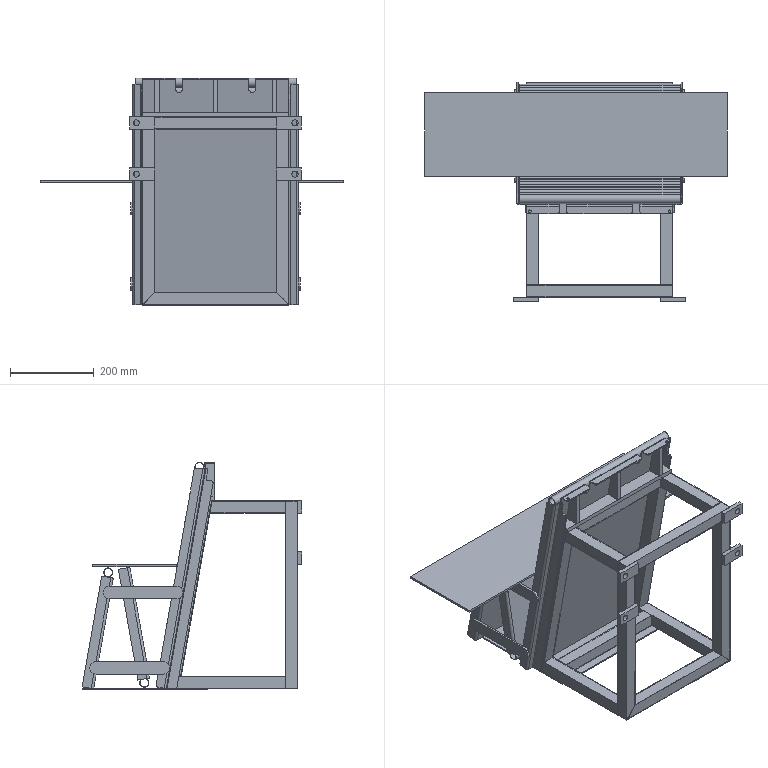Part | NX | features guide rail pipe_Default_As Machined_ 24, material feeder 3, material feeder support 3, pipe belum expand 2, pipe partition 2, stopper partition 2 | 81 solids | 519 faces | box 723 x 525.58 x 545.165 mm | volume 4966986 mm3 | plane 361 | cylinder 158 | commonest cylinder face diameters 19.8 x50 22.2 x50 10 x27 30 x8 4 x7 6 x4